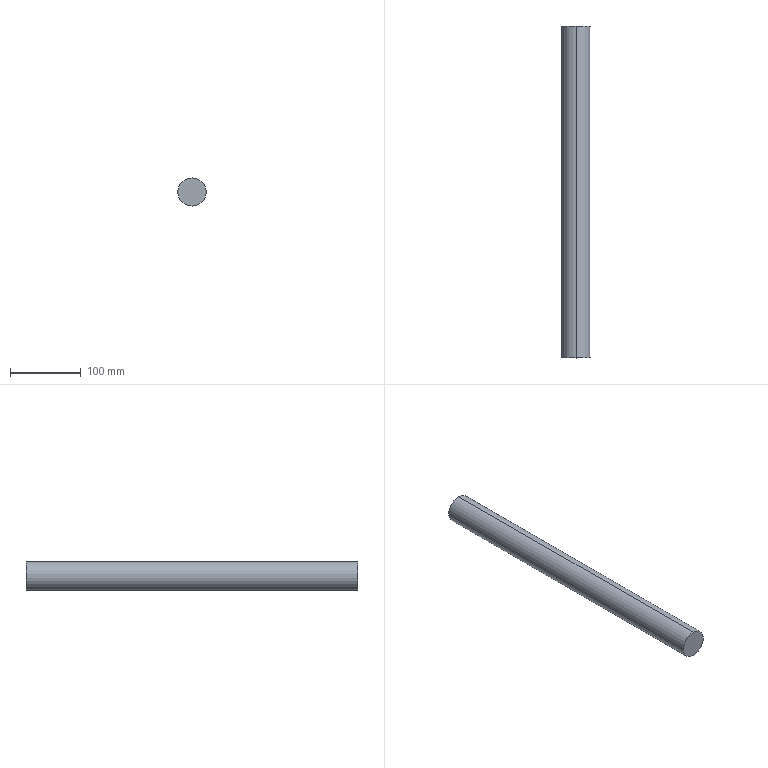Part | STEP file | PSFJ40-470 | 1 solid | 4 faces | box 40 x 470 x 40 mm | volume 590619 mm3 | cylinder 2 | plane 2 | commonest cylinder face diameters 40 x2
STEP:
#1=CARTESIAN_POINT('',(0.,0.,0.));
#2=DIRECTION('',(0.,0.,1.));
#3=DIRECTION('',(1.,0.,0.));
#4=AXIS2_PLACEMENT_3D('',#1,#2,#3);
#5=CARTESIAN_POINT('',(0.,470.,20.));
#6=VERTEX_POINT('',#5);
#7=CARTESIAN_POINT('',(0.,470.,-20.));
#8=VERTEX_POINT('',#7);
#9=CARTESIAN_POINT('',(0.,470.,0.));
#10=DIRECTION('',(0.,1.,0.));
#11=DIRECTION('',(0.,0.,1.));
#12=AXIS2_PLACEMENT_3D('',#9,#10,#11);
#13=CIRCLE('',#12,20.);
#14=CARTESIAN_POINT('',(0.,470.,0.));
#15=DIRECTION('',(0.,-1.,0.));
#16=DIRECTION('',(0.,0.,-1.));
#17=AXIS2_PLACEMENT_3D('',#14,#15,#16);
#18=CYLINDRICAL_SURFACE('',#17,20.);
#19=CARTESIAN_POINT('',(3.142,0.));
#20=DIRECTION('',(-1.,0.));
#21=VECTOR('',#20,1.);
#22=LINE('',#19,#21);
#23=(GEOMETRIC_REPRESENTATION_CONTEXT(2)PARAMETRIC_REPRESENTATION_CONTEXT()REPRESENTATION_CONTEXT('',''));
#24=DEFINITIONAL_REPRESENTATION('',(#22),#23);
#25=PCURVE('',#18,#24);
#26=CARTESIAN_POINT('',(0.,470.,0.));
#27=DIRECTION('',(0.,1.,0.));
#28=DIRECTION('',(0.,0.,1.));
#29=AXIS2_PLACEMENT_3D('',#26,#27,#28);
#30=PLANE('',#29);
#31=CARTESIAN_POINT('',(0.,0.));
#32=DIRECTION('',(1.,0.));
#33=AXIS2_PLACEMENT_2D('',#31,#32);
#34=CIRCLE('',#33,20.);
#35=(GEOMETRIC_REPRESENTATION_CONTEXT(2)PARAMETRIC_REPRESENTATION_CONTEXT()REPRESENTATION_CONTEXT('',''));
#36=DEFINITIONAL_REPRESENTATION('',(#34),#35);
#37=PCURVE('',#30,#36);
#38=SURFACE_CURVE('',#13,(#25,#37),.PCURVE_S1.);
#39=EDGE_CURVE('',#6,#8,#38,.T.);
#40=ORIENTED_EDGE('',*,*,#39,.F.);
#41=CARTESIAN_POINT('',(0.,0.,20.));
#42=VERTEX_POINT('',#41);
#43=CARTESIAN_POINT('',(0.,470.,20.));
#44=DIRECTION('',(0.,-1.,0.));
#45=VECTOR('',#44,1.);
#46=LINE('',#43,#45);
#47=CARTESIAN_POINT('',(3.142,0.));
#48=DIRECTION('',(0.,1.));
#49=VECTOR('',#48,1.);
#50=LINE('',#47,#49);
#51=(GEOMETRIC_REPRESENTATION_CONTEXT(2)PARAMETRIC_REPRESENTATION_CONTEXT()REPRESENTATION_CONTEXT('',''));
#52=DEFINITIONAL_REPRESENTATION('',(#50),#51);
#53=PCURVE('',#18,#52);
#54=CARTESIAN_POINT('',(0.,470.,0.));
#55=DIRECTION('',(0.,-1.,0.));
#56=DIRECTION('',(0.,0.,-1.));
#57=AXIS2_PLACEMENT_3D('',#54,#55,#56);
#58=CYLINDRICAL_SURFACE('',#57,20.);
#59=CARTESIAN_POINT('',(3.142,0.));
#60=DIRECTION('',(0.,1.));
#61=VECTOR('',#60,1.);
#62=LINE('',#59,#61);
#63=(GEOMETRIC_REPRESENTATION_CONTEXT(2)PARAMETRIC_REPRESENTATION_CONTEXT()REPRESENTATION_CONTEXT('',''));
#64=DEFINITIONAL_REPRESENTATION('',(#62),#63);
#65=PCURVE('',#58,#64);
#66=SURFACE_CURVE('',#46,(#53,#65),.PCURVE_S1.);
#67=EDGE_CURVE('',#6,#42,#66,.T.);
#68=ORIENTED_EDGE('',*,*,#67,.T.);
#69=CARTESIAN_POINT('',(0.,0.,-20.));
#70=VERTEX_POINT('',#69);
#71=CARTESIAN_POINT('',(0.,0.,0.));
#72=DIRECTION('',(0.,1.,0.));
#73=DIRECTION('',(0.,0.,1.));
#74=AXIS2_PLACEMENT_3D('',#71,#72,#73);
#75=CIRCLE('',#74,20.);
#76=CARTESIAN_POINT('',(3.142,470.));
#77=DIRECTION('',(-1.,0.));
#78=VECTOR('',#77,1.);
#79=LINE('',#76,#78);
#80=(GEOMETRIC_REPRESENTATION_CONTEXT(2)PARAMETRIC_REPRESENTATION_CONTEXT()REPRESENTATION_CONTEXT('',''));
#81=DEFINITIONAL_REPRESENTATION('',(#79),#80);
#82=PCURVE('',#18,#81);
#83=CARTESIAN_POINT('',(0.,0.,0.));
#84=DIRECTION('',(0.,1.,0.));
#85=DIRECTION('',(0.,0.,1.));
#86=AXIS2_PLACEMENT_3D('',#83,#84,#85);
#87=PLANE('',#86);
#88=CARTESIAN_POINT('',(0.,0.));
#89=DIRECTION('',(1.,0.));
#90=AXIS2_PLACEMENT_2D('',#88,#89);
#91=CIRCLE('',#90,20.);
#92=(GEOMETRIC_REPRESENTATION_CONTEXT(2)PARAMETRIC_REPRESENTATION_CONTEXT()REPRESENTATION_CONTEXT('',''));
#93=DEFINITIONAL_REPRESENTATION('',(#91),#92);
#94=PCURVE('',#87,#93);
#95=SURFACE_CURVE('',#75,(#82,#94),.PCURVE_S1.);
#96=EDGE_CURVE('',#42,#70,#95,.T.);
#97=ORIENTED_EDGE('',*,*,#96,.T.);
#98=CARTESIAN_POINT('',(0.,470.,-20.));
#99=DIRECTION('',(0.,-1.,0.));
#100=VECTOR('',#99,1.);
#101=LINE('',#98,#100);
#102=CARTESIAN_POINT('',(0.,0.));
#103=DIRECTION('',(0.,1.));
#104=VECTOR('',#103,1.);
#105=LINE('',#102,#104);
#106=(GEOMETRIC_REPRESENTATION_CONTEXT(2)PARAMETRIC_REPRESENTATION_CONTEXT()REPRESENTATION_CONTEXT('',''));
#107=DEFINITIONAL_REPRESENTATION('',(#105),#106);
#108=PCURVE('',#18,#107);
#109=CARTESIAN_POINT('',(6.283,0.));
#110=DIRECTION('',(0.,1.));
#111=VECTOR('',#110,1.);
#112=LINE('',#109,#111);
#113=(GEOMETRIC_REPRESENTATION_CONTEXT(2)PARAMETRIC_REPRESENTATION_CONTEXT()REPRESENTATION_CONTEXT('',''));
#114=DEFINITIONAL_REPRESENTATION('',(#112),#113);
#115=PCURVE('',#58,#114);
#116=SURFACE_CURVE('',#101,(#108,#115),.PCURVE_S1.);
#117=EDGE_CURVE('',#8,#70,#116,.T.);
#118=ORIENTED_EDGE('',*,*,#117,.F.);
#119=EDGE_LOOP('',(#40,#68,#97,#118));
#120=FACE_BOUND('',#119,.T.);
#121=ADVANCED_FACE('',(#120),#18,.T.);
#122=ORIENTED_EDGE('',*,*,#67,.F.);
#123=CARTESIAN_POINT('',(0.,470.,0.));
#124=DIRECTION('',(0.,1.,0.));
#125=DIRECTION('',(0.,0.,1.));
#126=AXIS2_PLACEMENT_3D('',#123,#124,#125);
#127=CIRCLE('',#126,20.);
#128=CARTESIAN_POINT('',(9.425,0.));
#129=DIRECTION('',(-1.,0.));
#130=VECTOR('',#129,1.);
#131=LINE('',#128,#130);
#132=(GEOMETRIC_REPRESENTATION_CONTEXT(2)PARAMETRIC_REPRESENTATION_CONTEXT()REPRESENTATION_CONTEXT('',''));
#133=DEFINITIONAL_REPRESENTATION('',(#131),#132);
#134=PCURVE('',#58,#133);
#135=CARTESIAN_POINT('',(0.,0.));
#136=DIRECTION('',(1.,0.));
#137=AXIS2_PLACEMENT_2D('',#135,#136);
#138=CIRCLE('',#137,20.);
#139=(GEOMETRIC_REPRESENTATION_CONTEXT(2)PARAMETRIC_REPRESENTATION_CONTEXT()REPRESENTATION_CONTEXT('',''));
#140=DEFINITIONAL_REPRESENTATION('',(#138),#139);
#141=PCURVE('',#30,#140);
#142=SURFACE_CURVE('',#127,(#134,#141),.PCURVE_S1.);
#143=EDGE_CURVE('',#8,#6,#142,.T.);
#144=ORIENTED_EDGE('',*,*,#143,.F.);
#145=ORIENTED_EDGE('',*,*,#117,.T.);
#146=CARTESIAN_POINT('',(0.,0.,0.));
#147=DIRECTION('',(0.,1.,0.));
#148=DIRECTION('',(0.,0.,1.));
#149=AXIS2_PLACEMENT_3D('',#146,#147,#148);
#150=CIRCLE('',#149,20.);
#151=CARTESIAN_POINT('',(9.425,470.));
#152=DIRECTION('',(-1.,0.));
#153=VECTOR('',#152,1.);
#154=LINE('',#151,#153);
#155=(GEOMETRIC_REPRESENTATION_CONTEXT(2)PARAMETRIC_REPRESENTATION_CONTEXT()REPRESENTATION_CONTEXT('',''));
#156=DEFINITIONAL_REPRESENTATION('',(#154),#155);
#157=PCURVE('',#58,#156);
#158=CARTESIAN_POINT('',(0.,0.));
#159=DIRECTION('',(1.,0.));
#160=AXIS2_PLACEMENT_2D('',#158,#159);
#161=CIRCLE('',#160,20.);
#162=(GEOMETRIC_REPRESENTATION_CONTEXT(2)PARAMETRIC_REPRESENTATION_CONTEXT()REPRESENTATION_CONTEXT('',''));
#163=DEFINITIONAL_REPRESENTATION('',(#161),#162);
#164=PCURVE('',#87,#163);
#165=SURFACE_CURVE('',#150,(#157,#164),.PCURVE_S1.);
#166=EDGE_CURVE('',#70,#42,#165,.T.);
#167=ORIENTED_EDGE('',*,*,#166,.T.);
#168=EDGE_LOOP('',(#122,#144,#145,#167));
#169=FACE_BOUND('',#168,.T.);
#170=ADVANCED_FACE('',(#169),#58,.T.);
#171=ORIENTED_EDGE('',*,*,#143,.T.);
#172=ORIENTED_EDGE('',*,*,#39,.T.);
#173=EDGE_LOOP('',(#171,#172));
#174=FACE_BOUND('',#173,.T.);
#175=ADVANCED_FACE('',(#174),#30,.T.);
#176=ORIENTED_EDGE('',*,*,#166,.F.);
#177=ORIENTED_EDGE('',*,*,#96,.F.);
#178=EDGE_LOOP('',(#176,#177));
#179=FACE_BOUND('',#178,.T.);
#180=ADVANCED_FACE('',(#179),#87,.F.);
#181=CLOSED_SHELL('',(#121,#170,#175,#180));
#182=MANIFOLD_SOLID_BREP('',#181);
#183=(LENGTH_UNIT()NAMED_UNIT(*)SI_UNIT(.MILLI.,.METRE.));
#184=UNCERTAINTY_MEASURE_WITH_UNIT(LENGTH_MEASURE(0.0000001),#183,'','');
#185=(NAMED_UNIT(*)PLANE_ANGLE_UNIT()SI_UNIT($,.RADIAN.));
#186=(NAMED_UNIT(*)SI_UNIT($,.STERADIAN.)SOLID_ANGLE_UNIT());
#187=(GEOMETRIC_REPRESENTATION_CONTEXT(3)GLOBAL_UNCERTAINTY_ASSIGNED_CONTEXT((#184))GLOBAL_UNIT_ASSIGNED_CONTEXT((#183,#185,#186))REPRESENTATION_CONTEXT('',''));
#188=ADVANCED_BREP_SHAPE_REPRESENTATION('',(#4,#182),#187);